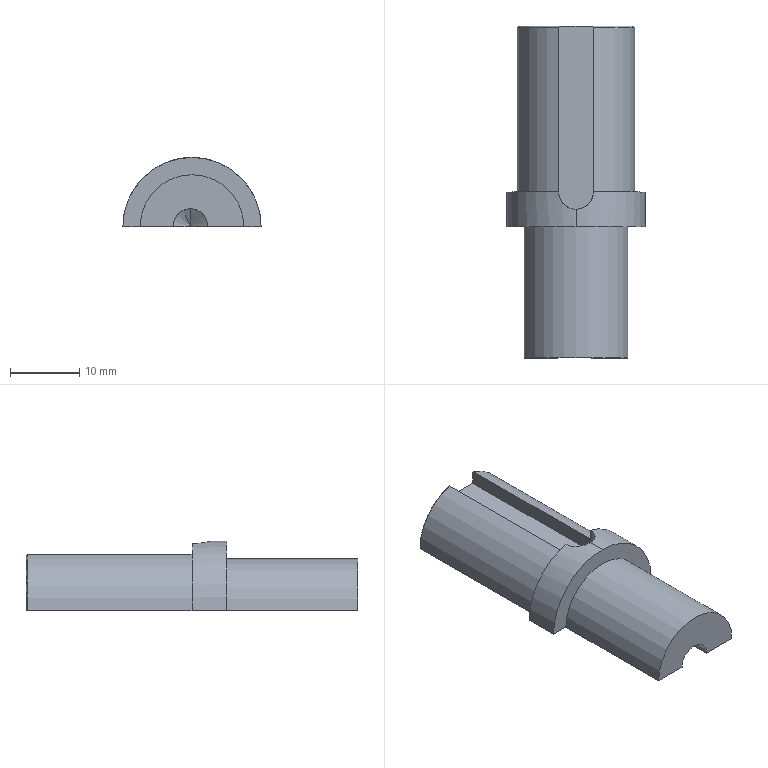Part | STEP file | Cuon T phu H01_9 | 1 solid | 24 faces | box 20 x 48 x 10 mm | volume 4554 mm3 | cylinder 9 | plane 9 | cone 6 | commonest cylinder face diameters 5 x4 17 x2 20 x2 15 x1